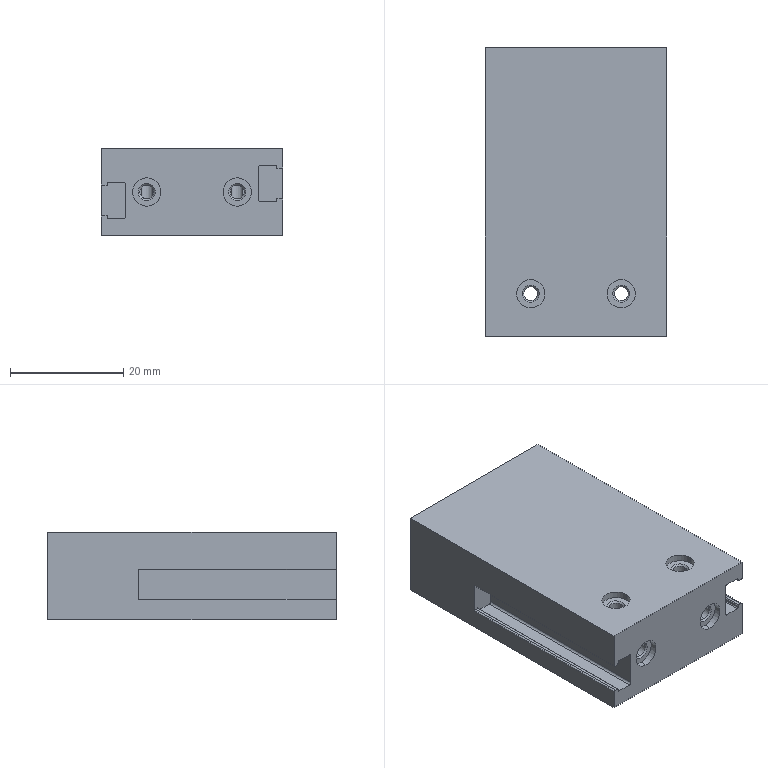Part | STEP file | PN_0047 | 1 solid | 96 faces | box 32 x 51 x 15.5 mm | volume 23128 mm3 | cylinder 46 | plane 34 | cone 16 | commonest cylinder face diameters 2.459 x18 5 x12 0.4 x8 0.8 x8